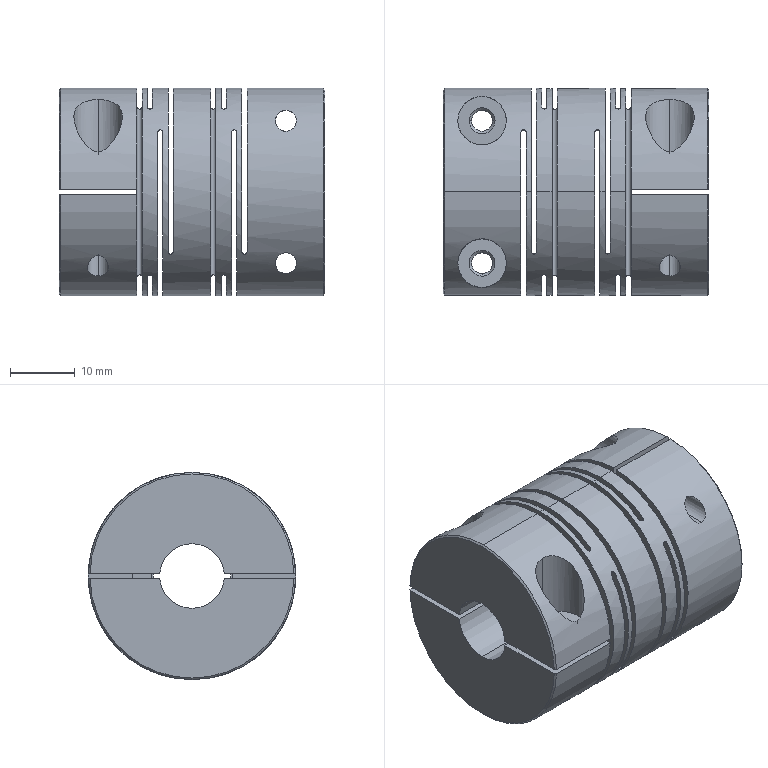Part | STEP file | 0230_Z_008_CPLCN32-10-12_1 | 1 solid | 109 faces | box 41 x 32 x 32 mm | volume 22644 mm3 | cylinder 60 | plane 36 | cone 13 | commonest cylinder face diameters 12.5 x14 0.8 x10 3.242 x8 4 x8 7.5 x8 32 x7